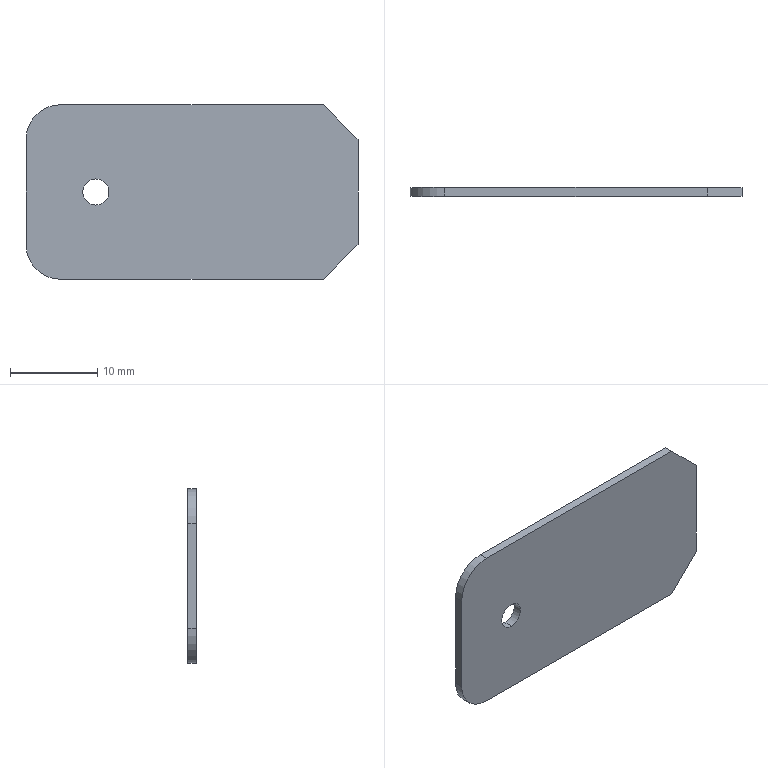Part | STEP file | RJWD-DY-0108_0003 | 1 solid | 12 faces | box 38 x 1 x 20 mm | volume 730.064 mm3 | plane 8 | cylinder 4 | commonest cylinder face diameters 3 x2 8 x2
STEP:
#1=CARTESIAN_POINT('',(0.,0.,0.));
#2=DIRECTION('',(0.,0.,1.));
#3=DIRECTION('',(1.,0.,0.));
#4=AXIS2_PLACEMENT_3D('',#1,#2,#3);
#5=CARTESIAN_POINT('',(231.,4571.8,302.644));
#6=VERTEX_POINT('',#5);
#7=CARTESIAN_POINT('',(231.,4571.8,314.644));
#8=VERTEX_POINT('',#7);
#9=CARTESIAN_POINT('',(231.,4571.8,302.644));
#10=DIRECTION('',(0.,0.,1.));
#11=VECTOR('',#10,1.);
#12=LINE('',#9,#11);
#13=CARTESIAN_POINT('',(231.,4571.8,298.644));
#14=DIRECTION('',(-1.,0.,0.));
#15=DIRECTION('',(0.,0.,-1.));
#16=AXIS2_PLACEMENT_3D('',#13,#14,#15);
#17=PLANE('',#16);
#18=CARTESIAN_POINT('',(-4.,0.));
#19=DIRECTION('',(-1.,0.));
#20=VECTOR('',#19,1.);
#21=LINE('',#18,#20);
#22=(GEOMETRIC_REPRESENTATION_CONTEXT(2)PARAMETRIC_REPRESENTATION_CONTEXT()REPRESENTATION_CONTEXT('',''));
#23=DEFINITIONAL_REPRESENTATION('',(#21),#22);
#24=PCURVE('',#17,#23);
#25=CARTESIAN_POINT('',(195.,4571.8,314.644));
#26=DIRECTION('',(0.,1.,0.));
#27=DIRECTION('',(0.,0.,1.));
#28=AXIS2_PLACEMENT_3D('',#25,#26,#27);
#29=PLANE('',#28);
#30=CARTESIAN_POINT('',(-12.,36.));
#31=DIRECTION('',(1.,0.));
#32=VECTOR('',#31,1.);
#33=LINE('',#30,#32);
#34=(GEOMETRIC_REPRESENTATION_CONTEXT(2)PARAMETRIC_REPRESENTATION_CONTEXT()REPRESENTATION_CONTEXT('',''));
#35=DEFINITIONAL_REPRESENTATION('',(#33),#34);
#36=PCURVE('',#29,#35);
#37=SURFACE_CURVE('',#12,(#24,#36),.PCURVE_S1.);
#38=EDGE_CURVE('',#6,#8,#37,.T.);
#39=ORIENTED_EDGE('',*,*,#38,.F.);
#40=CARTESIAN_POINT('',(231.,4570.8,302.644));
#41=VERTEX_POINT('',#40);
#42=CARTESIAN_POINT('',(231.,4571.8,302.644));
#43=DIRECTION('',(0.,-1.,0.));
#44=VECTOR('',#43,1.);
#45=LINE('',#42,#44);
#46=CARTESIAN_POINT('',(-4.,0.));
#47=DIRECTION('',(0.,1.));
#48=VECTOR('',#47,1.);
#49=LINE('',#46,#48);
#50=(GEOMETRIC_REPRESENTATION_CONTEXT(2)PARAMETRIC_REPRESENTATION_CONTEXT()REPRESENTATION_CONTEXT('',''));
#51=DEFINITIONAL_REPRESENTATION('',(#49),#50);
#52=PCURVE('',#17,#51);
#53=CARTESIAN_POINT('',(231.,4571.8,302.644));
#54=DIRECTION('',(-0.7071,0.,0.7071));
#55=DIRECTION('',(0.,-1.,0.));
#56=AXIS2_PLACEMENT_3D('',#53,#54,#55);
#57=PLANE('',#56);
#58=CARTESIAN_POINT('',(0.,0.));
#59=DIRECTION('',(1.,0.));
#60=VECTOR('',#59,1.);
#61=LINE('',#58,#60);
#62=(GEOMETRIC_REPRESENTATION_CONTEXT(2)PARAMETRIC_REPRESENTATION_CONTEXT()REPRESENTATION_CONTEXT('',''));
#63=DEFINITIONAL_REPRESENTATION('',(#61),#62);
#64=PCURVE('',#57,#63);
#65=SURFACE_CURVE('',#45,(#52,#64),.PCURVE_S1.);
#66=EDGE_CURVE('',#6,#41,#65,.T.);
#67=ORIENTED_EDGE('',*,*,#66,.T.);
#68=CARTESIAN_POINT('',(231.,4570.8,314.644));
#69=VERTEX_POINT('',#68);
#70=CARTESIAN_POINT('',(231.,4570.8,302.644));
#71=DIRECTION('',(0.,0.,1.));
#72=VECTOR('',#71,1.);
#73=LINE('',#70,#72);
#74=CARTESIAN_POINT('',(-4.,1.));
#75=DIRECTION('',(-1.,0.));
#76=VECTOR('',#75,1.);
#77=LINE('',#74,#76);
#78=(GEOMETRIC_REPRESENTATION_CONTEXT(2)PARAMETRIC_REPRESENTATION_CONTEXT()REPRESENTATION_CONTEXT('',''));
#79=DEFINITIONAL_REPRESENTATION('',(#77),#78);
#80=PCURVE('',#17,#79);
#81=CARTESIAN_POINT('',(195.,4570.8,314.644));
#82=DIRECTION('',(0.,1.,0.));
#83=DIRECTION('',(0.,0.,1.));
#84=AXIS2_PLACEMENT_3D('',#81,#82,#83);
#85=PLANE('',#84);
#86=CARTESIAN_POINT('',(-12.,36.));
#87=DIRECTION('',(1.,0.));
#88=VECTOR('',#87,1.);
#89=LINE('',#86,#88);
#90=(GEOMETRIC_REPRESENTATION_CONTEXT(2)PARAMETRIC_REPRESENTATION_CONTEXT()REPRESENTATION_CONTEXT('',''));
#91=DEFINITIONAL_REPRESENTATION('',(#89),#90);
#92=PCURVE('',#85,#91);
#93=SURFACE_CURVE('',#73,(#80,#92),.PCURVE_S1.);
#94=EDGE_CURVE('',#41,#69,#93,.T.);
#95=ORIENTED_EDGE('',*,*,#94,.T.);
#96=CARTESIAN_POINT('',(231.,4570.8,314.644));
#97=DIRECTION('',(0.,1.,0.));
#98=VECTOR('',#97,1.);
#99=LINE('',#96,#98);
#100=CARTESIAN_POINT('',(-16.,1.));
#101=DIRECTION('',(0.,-1.));
#102=VECTOR('',#101,1.);
#103=LINE('',#100,#102);
#104=(GEOMETRIC_REPRESENTATION_CONTEXT(2)PARAMETRIC_REPRESENTATION_CONTEXT()REPRESENTATION_CONTEXT('',''));
#105=DEFINITIONAL_REPRESENTATION('',(#103),#104);
#106=PCURVE('',#17,#105);
#107=CARTESIAN_POINT('',(227.,4571.8,318.644));
#108=DIRECTION('',(-0.7071,0.,-0.7071));
#109=DIRECTION('',(0.,-1.,0.));
#110=AXIS2_PLACEMENT_3D('',#107,#108,#109);
#111=PLANE('',#110);
#112=CARTESIAN_POINT('',(1.,-5.657));
#113=DIRECTION('',(-1.,0.));
#114=VECTOR('',#113,1.);
#115=LINE('',#112,#114);
#116=(GEOMETRIC_REPRESENTATION_CONTEXT(2)PARAMETRIC_REPRESENTATION_CONTEXT()REPRESENTATION_CONTEXT('',''));
#117=DEFINITIONAL_REPRESENTATION('',(#115),#116);
#118=PCURVE('',#111,#117);
#119=SURFACE_CURVE('',#99,(#106,#118),.PCURVE_S1.);
#120=EDGE_CURVE('',#69,#8,#119,.T.);
#121=ORIENTED_EDGE('',*,*,#120,.T.);
#122=EDGE_LOOP('',(#39,#67,#95,#121));
#123=FACE_BOUND('',#122,.F.);
#124=ADVANCED_FACE('',(#123),#17,.F.);
#125=CARTESIAN_POINT('',(193.,4571.8,314.644));
#126=VERTEX_POINT('',#125);
#127=CARTESIAN_POINT('',(197.,4571.8,318.644));
#128=VERTEX_POINT('',#127);
#129=CARTESIAN_POINT('',(197.,4571.8,314.644));
#130=DIRECTION('',(0.,1.,0.));
#131=DIRECTION('',(-1.,0.,0.));
#132=AXIS2_PLACEMENT_3D('',#129,#130,#131);
#133=CIRCLE('',#132,4.);
#134=CARTESIAN_POINT('',(0.,2.));
#135=DIRECTION('',(0.,-1.));
#136=AXIS2_PLACEMENT_2D('',#134,#135);
#137=CIRCLE('',#136,4.);
#138=(GEOMETRIC_REPRESENTATION_CONTEXT(2)PARAMETRIC_REPRESENTATION_CONTEXT()REPRESENTATION_CONTEXT('',''));
#139=DEFINITIONAL_REPRESENTATION('',(#137),#138);
#140=PCURVE('',#29,#139);
#141=CARTESIAN_POINT('',(197.,4576.711,314.644));
#142=DIRECTION('',(0.,-1.,0.));
#143=DIRECTION('',(0.,0.,1.));
#144=AXIS2_PLACEMENT_3D('',#141,#142,#143);
#145=CYLINDRICAL_SURFACE('',#144,4.);
#146=CARTESIAN_POINT('',(1.571,4.911));
#147=DIRECTION('',(-1.,0.));
#148=VECTOR('',#147,1.);
#149=LINE('',#146,#148);
#150=(GEOMETRIC_REPRESENTATION_CONTEXT(2)PARAMETRIC_REPRESENTATION_CONTEXT()REPRESENTATION_CONTEXT('',''));
#151=DEFINITIONAL_REPRESENTATION('',(#149),#150);
#152=PCURVE('',#145,#151);
#153=SURFACE_CURVE('',#133,(#140,#152),.PCURVE_S1.);
#154=EDGE_CURVE('',#126,#128,#153,.T.);
#155=ORIENTED_EDGE('',*,*,#154,.F.);
#156=CARTESIAN_POINT('',(193.,4571.8,302.644));
#157=VERTEX_POINT('',#156);
#158=CARTESIAN_POINT('',(193.,4571.8,314.644));
#159=DIRECTION('',(0.,0.,-1.));
#160=VECTOR('',#159,1.);
#161=LINE('',#158,#160);
#162=CARTESIAN_POINT('',(0.,-2.));
#163=DIRECTION('',(-1.,0.));
#164=VECTOR('',#163,1.);
#165=LINE('',#162,#164);
#166=(GEOMETRIC_REPRESENTATION_CONTEXT(2)PARAMETRIC_REPRESENTATION_CONTEXT()REPRESENTATION_CONTEXT('',''));
#167=DEFINITIONAL_REPRESENTATION('',(#165),#166);
#168=PCURVE('',#29,#167);
#169=CARTESIAN_POINT('',(193.,4571.8,314.644));
#170=DIRECTION('',(1.,0.,0.));
#171=DIRECTION('',(0.,0.,1.));
#172=AXIS2_PLACEMENT_3D('',#169,#170,#171);
#173=PLANE('',#172);
#174=CARTESIAN_POINT('',(0.,0.));
#175=DIRECTION('',(-1.,0.));
#176=VECTOR('',#175,1.);
#177=LINE('',#174,#176);
#178=(GEOMETRIC_REPRESENTATION_CONTEXT(2)PARAMETRIC_REPRESENTATION_CONTEXT()REPRESENTATION_CONTEXT('',''));
#179=DEFINITIONAL_REPRESENTATION('',(#177),#178);
#180=PCURVE('',#173,#179);
#181=SURFACE_CURVE('',#161,(#168,#180),.PCURVE_S1.);
#182=EDGE_CURVE('',#126,#157,#181,.T.);
#183=ORIENTED_EDGE('',*,*,#182,.T.);
#184=CARTESIAN_POINT('',(197.,4571.8,298.644));
#185=VERTEX_POINT('',#184);
#186=CARTESIAN_POINT('',(197.,4571.8,302.644));
#187=DIRECTION('',(0.,1.,0.));
#188=DIRECTION('',(0.,0.,-1.));
#189=AXIS2_PLACEMENT_3D('',#186,#187,#188);
#190=CIRCLE('',#189,4.);
#191=CARTESIAN_POINT('',(-12.,2.));
#192=DIRECTION('',(-1.,0.));
#193=AXIS2_PLACEMENT_2D('',#191,#192);
#194=CIRCLE('',#193,4.);
#195=(GEOMETRIC_REPRESENTATION_CONTEXT(2)PARAMETRIC_REPRESENTATION_CONTEXT()REPRESENTATION_CONTEXT('',''));
#196=DEFINITIONAL_REPRESENTATION('',(#194),#195);
#197=PCURVE('',#29,#196);
#198=CARTESIAN_POINT('',(197.,4576.711,302.644));
#199=DIRECTION('',(0.,-1.,0.));
#200=DIRECTION('',(-1.,0.,0.));
#201=AXIS2_PLACEMENT_3D('',#198,#199,#200);
#202=CYLINDRICAL_SURFACE('',#201,4.);
#203=CARTESIAN_POINT('',(1.571,4.911));
#204=DIRECTION('',(-1.,0.));
#205=VECTOR('',#204,1.);
#206=LINE('',#203,#205);
#207=(GEOMETRIC_REPRESENTATION_CONTEXT(2)PARAMETRIC_REPRESENTATION_CONTEXT()REPRESENTATION_CONTEXT('',''));
#208=DEFINITIONAL_REPRESENTATION('',(#206),#207);
#209=PCURVE('',#202,#208);
#210=SURFACE_CURVE('',#190,(#197,#209),.PCURVE_S1.);
#211=EDGE_CURVE('',#185,#157,#210,.T.);
#212=ORIENTED_EDGE('',*,*,#211,.F.);
#213=CARTESIAN_POINT('',(227.,4571.8,298.644));
#214=VERTEX_POINT('',#213);
#215=CARTESIAN_POINT('',(227.,4571.8,298.644));
#216=DIRECTION('',(-1.,0.,0.));
#217=VECTOR('',#216,1.);
#218=LINE('',#215,#217);
#219=CARTESIAN_POINT('',(-16.,32.));
#220=DIRECTION('',(0.,-1.));
#221=VECTOR('',#220,1.);
#222=LINE('',#219,#221);
#223=(GEOMETRIC_REPRESENTATION_CONTEXT(2)PARAMETRIC_REPRESENTATION_CONTEXT()REPRESENTATION_CONTEXT('',''));
#224=DEFINITIONAL_REPRESENTATION('',(#222),#223);
#225=PCURVE('',#29,#224);
#226=CARTESIAN_POINT('',(195.,4571.8,298.644));
#227=DIRECTION('',(0.,0.,1.));
#228=DIRECTION('',(-1.,0.,0.));
#229=AXIS2_PLACEMENT_3D('',#226,#227,#228);
#230=PLANE('',#229);
#231=CARTESIAN_POINT('',(-32.,0.));
#232=DIRECTION('',(1.,0.));
#233=VECTOR('',#232,1.);
#234=LINE('',#231,#233);
#235=(GEOMETRIC_REPRESENTATION_CONTEXT(2)PARAMETRIC_REPRESENTATION_CONTEXT()REPRESENTATION_CONTEXT('',''));
#236=DEFINITIONAL_REPRESENTATION('',(#234),#235);
#237=PCURVE('',#230,#236);
#238=SURFACE_CURVE('',#218,(#225,#237),.PCURVE_S1.);
#239=EDGE_CURVE('',#214,#185,#238,.T.);
#240=ORIENTED_EDGE('',*,*,#239,.F.);
#241=CARTESIAN_POINT('',(231.,4571.8,302.644));
#242=DIRECTION('',(-0.7071,0.,-0.7071));
#243=VECTOR('',#242,1.);
#244=LINE('',#241,#243);
#245=CARTESIAN_POINT('',(-12.,36.));
#246=DIRECTION('',(-0.7071,-0.7071));
#247=VECTOR('',#246,1.);
#248=LINE('',#245,#247);
#249=(GEOMETRIC_REPRESENTATION_CONTEXT(2)PARAMETRIC_REPRESENTATION_CONTEXT()REPRESENTATION_CONTEXT('',''));
#250=DEFINITIONAL_REPRESENTATION('',(#248),#249);
#251=PCURVE('',#29,#250);
#252=CARTESIAN_POINT('',(0.,0.));
#253=DIRECTION('',(0.,-1.));
#254=VECTOR('',#253,1.);
#255=LINE('',#252,#254);
#256=(GEOMETRIC_REPRESENTATION_CONTEXT(2)PARAMETRIC_REPRESENTATION_CONTEXT()REPRESENTATION_CONTEXT('',''));
#257=DEFINITIONAL_REPRESENTATION('',(#255),#256);
#258=PCURVE('',#57,#257);
#259=SURFACE_CURVE('',#244,(#251,#258),.PCURVE_S1.);
#260=EDGE_CURVE('',#6,#214,#259,.T.);
#261=ORIENTED_EDGE('',*,*,#260,.F.);
#262=ORIENTED_EDGE('',*,*,#38,.T.);
#263=CARTESIAN_POINT('',(227.,4571.8,318.644));
#264=VERTEX_POINT('',#263);
#265=CARTESIAN_POINT('',(227.,4571.8,318.644));
#266=DIRECTION('',(0.7071,0.,-0.7071));
#267=VECTOR('',#266,1.);
#268=LINE('',#265,#267);
#269=CARTESIAN_POINT('',(4.,32.));
#270=DIRECTION('',(-0.7071,0.7071));
#271=VECTOR('',#270,1.);
#272=LINE('',#269,#271);
#273=(GEOMETRIC_REPRESENTATION_CONTEXT(2)PARAMETRIC_REPRESENTATION_CONTEXT()REPRESENTATION_CONTEXT('',''));
#274=DEFINITIONAL_REPRESENTATION('',(#272),#273);
#275=PCURVE('',#29,#274);
#276=CARTESIAN_POINT('',(0.,0.));
#277=DIRECTION('',(0.,-1.));
#278=VECTOR('',#277,1.);
#279=LINE('',#276,#278);
#280=(GEOMETRIC_REPRESENTATION_CONTEXT(2)PARAMETRIC_REPRESENTATION_CONTEXT()REPRESENTATION_CONTEXT('',''));
#281=DEFINITIONAL_REPRESENTATION('',(#279),#280);
#282=PCURVE('',#111,#281);
#283=SURFACE_CURVE('',#268,(#275,#282),.PCURVE_S1.);
#284=EDGE_CURVE('',#264,#8,#283,.T.);
#285=ORIENTED_EDGE('',*,*,#284,.F.);
#286=CARTESIAN_POINT('',(197.,4571.8,318.644));
#287=DIRECTION('',(1.,0.,0.));
#288=VECTOR('',#287,1.);
#289=LINE('',#286,#288);
#290=CARTESIAN_POINT('',(4.,2.));
#291=DIRECTION('',(0.,1.));
#292=VECTOR('',#291,1.);
#293=LINE('',#290,#292);
#294=(GEOMETRIC_REPRESENTATION_CONTEXT(2)PARAMETRIC_REPRESENTATION_CONTEXT()REPRESENTATION_CONTEXT('',''));
#295=DEFINITIONAL_REPRESENTATION('',(#293),#294);
#296=PCURVE('',#29,#295);
#297=CARTESIAN_POINT('',(231.,4571.8,318.644));
#298=DIRECTION('',(0.,0.,-1.));
#299=DIRECTION('',(1.,0.,0.));
#300=AXIS2_PLACEMENT_3D('',#297,#298,#299);
#301=PLANE('',#300);
#302=CARTESIAN_POINT('',(-34.,0.));
#303=DIRECTION('',(1.,0.));
#304=VECTOR('',#303,1.);
#305=LINE('',#302,#304);
#306=(GEOMETRIC_REPRESENTATION_CONTEXT(2)PARAMETRIC_REPRESENTATION_CONTEXT()REPRESENTATION_CONTEXT('',''));
#307=DEFINITIONAL_REPRESENTATION('',(#305),#306);
#308=PCURVE('',#301,#307);
#309=SURFACE_CURVE('',#289,(#296,#308),.PCURVE_S1.);
#310=EDGE_CURVE('',#128,#264,#309,.T.);
#311=ORIENTED_EDGE('',*,*,#310,.F.);
#312=EDGE_LOOP('',(#155,#183,#212,#240,#261,#262,#285,#311));
#313=FACE_BOUND('',#312,.F.);
#314=CARTESIAN_POINT('',(200.999,4571.8,310.144));
#315=VERTEX_POINT('',#314);
#316=CARTESIAN_POINT('',(200.999,4571.8,307.144));
#317=VERTEX_POINT('',#316);
#318=CARTESIAN_POINT('',(200.999,4571.8,308.644));
#319=DIRECTION('',(0.,1.,0.));
#320=DIRECTION('',(0.,0.,1.));
#321=AXIS2_PLACEMENT_3D('',#318,#319,#320);
#322=CIRCLE('',#321,1.5);
#323=CARTESIAN_POINT('',(-6.,5.999));
#324=DIRECTION('',(1.,0.));
#325=AXIS2_PLACEMENT_2D('',#323,#324);
#326=CIRCLE('',#325,1.5);
#327=(GEOMETRIC_REPRESENTATION_CONTEXT(2)PARAMETRIC_REPRESENTATION_CONTEXT()REPRESENTATION_CONTEXT('',''));
#328=DEFINITIONAL_REPRESENTATION('',(#326),#327);
#329=PCURVE('',#29,#328);
#330=CARTESIAN_POINT('',(200.999,4571.8,308.644));
#331=DIRECTION('',(0.,-1.,0.));
#332=DIRECTION('',(0.,0.,-1.));
#333=AXIS2_PLACEMENT_3D('',#330,#331,#332);
#334=CYLINDRICAL_SURFACE('',#333,1.5);
#335=CARTESIAN_POINT('',(3.142,0.));
#336=DIRECTION('',(-1.,0.));
#337=VECTOR('',#336,1.);
#338=LINE('',#335,#337);
#339=(GEOMETRIC_REPRESENTATION_CONTEXT(2)PARAMETRIC_REPRESENTATION_CONTEXT()REPRESENTATION_CONTEXT('',''));
#340=DEFINITIONAL_REPRESENTATION('',(#338),#339);
#341=PCURVE('',#334,#340);
#342=SURFACE_CURVE('',#322,(#329,#341),.PCURVE_S1.);
#343=EDGE_CURVE('',#315,#317,#342,.T.);
#344=ORIENTED_EDGE('',*,*,#343,.T.);
#345=CARTESIAN_POINT('',(200.999,4571.8,308.644));
#346=DIRECTION('',(0.,-1.,0.));
#347=DIRECTION('',(0.,0.,1.));
#348=AXIS2_PLACEMENT_3D('',#345,#346,#347);
#349=CIRCLE('',#348,1.5);
#350=CARTESIAN_POINT('',(-4.5,5.999));
#351=CARTESIAN_POINT('',(-4.5,3.401));
#352=CARTESIAN_POINT('',(-6.75,4.7));
#353=CARTESIAN_POINT('',(-9.,5.999));
#354=CARTESIAN_POINT('',(-6.75,7.298));
#355=CARTESIAN_POINT('',(-4.5,8.597));
#356=CARTESIAN_POINT('',(-4.5,5.999));
#357=(BOUNDED_CURVE()B_SPLINE_CURVE(2,(#350,#351,#352,#353,#354,#355,#356),.UNSPECIFIED.,.T.,.F.)B_SPLINE_CURVE_WITH_KNOTS((1,2,2,2,2,1),(-2.094,0.,2.094,4.189,6.283,8.378),.UNSPECIFIED.)CURVE()GEOMETRIC_REPRESENTATION_ITEM()RATIONAL_B_SPLINE_CURVE((1.,0.5,1.,0.5,1.,0.5,1.))REPRESENTATION_ITEM(''));
#358=(GEOMETRIC_REPRESENTATION_CONTEXT(2)PARAMETRIC_REPRESENTATION_CONTEXT()REPRESENTATION_CONTEXT('',''));
#359=DEFINITIONAL_REPRESENTATION('',(#357),#358);
#360=PCURVE('',#29,#359);
#361=CARTESIAN_POINT('',(200.999,4571.8,308.644));
#362=DIRECTION('',(0.,-1.,0.));
#363=DIRECTION('',(0.,0.,-1.));
#364=AXIS2_PLACEMENT_3D('',#361,#362,#363);
#365=CYLINDRICAL_SURFACE('',#364,1.5);
#366=CARTESIAN_POINT('',(3.142,0.));
#367=DIRECTION('',(1.,0.));
#368=VECTOR('',#367,1.);
#369=LINE('',#366,#368);
#370=(GEOMETRIC_REPRESENTATION_CONTEXT(2)PARAMETRIC_REPRESENTATION_CONTEXT()REPRESENTATION_CONTEXT('',''));
#371=DEFINITIONAL_REPRESENTATION('',(#369),#370);
#372=PCURVE('',#365,#371);
#373=SURFACE_CURVE('',#349,(#360,#372),.PCURVE_S1.);
#374=EDGE_CURVE('',#315,#317,#373,.T.);
#375=ORIENTED_EDGE('',*,*,#374,.F.);
#376=EDGE_LOOP('',(#344,#375));
#377=FACE_BOUND('',#376,.F.);
#378=ADVANCED_FACE('',(#313,#377),#29,.T.);
#379=ORIENTED_EDGE('',*,*,#343,.F.);
#380=CARTESIAN_POINT('',(200.999,4570.8,310.144));
#381=VERTEX_POINT('',#380);
#382=CARTESIAN_POINT('',(200.999,4571.8,310.144));
#383=DIRECTION('',(0.,-1.,0.));
#384=VECTOR('',#383,1.);
#385=LINE('',#382,#384);
#386=CARTESIAN_POINT('',(3.142,0.));
#387=DIRECTION('',(0.,1.));
#388=VECTOR('',#387,1.);
#389=LINE('',#386,#388);
#390=(GEOMETRIC_REPRESENTATION_CONTEXT(2)PARAMETRIC_REPRESENTATION_CONTEXT()REPRESENTATION_CONTEXT('',''));
#391=DEFINITIONAL_REPRESENTATION('',(#389),#390);
#392=PCURVE('',#334,#391);
#393=CARTESIAN_POINT('',(3.142,0.));
#394=DIRECTION('',(0.,1.));
#395=VECTOR('',#394,1.);
#396=LINE('',#393,#395);
#397=(GEOMETRIC_REPRESENTATION_CONTEXT(2)PARAMETRIC_REPRESENTATION_CONTEXT()REPRESENTATION_CONTEXT('',''));
#398=DEFINITIONAL_REPRESENTATION('',(#396),#397);
#399=PCURVE('',#365,#398);
#400=SURFACE_CURVE('',#385,(#392,#399),.PCURVE_S1.);
#401=EDGE_CURVE('',#315,#381,#400,.T.);
#402=ORIENTED_EDGE('',*,*,#401,.T.);
#403=CARTESIAN_POINT('',(200.999,4570.8,307.144));
#404=VERTEX_POINT('',#403);
#405=CARTESIAN_POINT('',(200.999,4570.8,308.644));
#406=DIRECTION('',(0.,-1.,0.));
#407=DIRECTION('',(0.,0.,-1.));
#408=AXIS2_PLACEMENT_3D('',#405,#406,#407);
#409=CIRCLE('',#408,1.5);
#410=CARTESIAN_POINT('',(0.,1.));
#411=DIRECTION('',(1.,0.));
#412=VECTOR('',#411,1.);
#413=LINE('',#410,#412);
#414=(GEOMETRIC_REPRESENTATION_CONTEXT(2)PARAMETRIC_REPRESENTATION_CONTEXT()REPRESENTATION_CONTEXT('',''));
#415=DEFINITIONAL_REPRESENTATION('',(#413),#414);
#416=PCURVE('',#334,#415);
#417=CARTESIAN_POINT('',(-7.5,5.999));
#418=CARTESIAN_POINT('',(-7.5,8.597));
#419=CARTESIAN_POINT('',(-5.25,7.298));
#420=CARTESIAN_POINT('',(-3.,5.999));
#421=CARTESIAN_POINT('',(-5.25,4.7));
#422=CARTESIAN_POINT('',(-7.5,3.401));
#423=CARTESIAN_POINT('',(-7.5,5.999));
#424=(BOUNDED_CURVE()B_SPLINE_CURVE(2,(#417,#418,#419,#420,#421,#422,#423),.UNSPECIFIED.,.T.,.F.)B_SPLINE_CURVE_WITH_KNOTS((1,2,2,2,2,1),(-2.094,0.,2.094,4.189,6.283,8.378),.UNSPECIFIED.)CURVE()GEOMETRIC_REPRESENTATION_ITEM()RATIONAL_B_SPLINE_CURVE((1.,0.5,1.,0.5,1.,0.5,1.))REPRESENTATION_ITEM(''));
#425=(GEOMETRIC_REPRESENTATION_CONTEXT(2)PARAMETRIC_REPRESENTATION_CONTEXT()REPRESENTATION_CONTEXT('',''));
#426=DEFINITIONAL_REPRESENTATION('',(#424),#425);
#427=PCURVE('',#85,#426);
#428=SURFACE_CURVE('',#409,(#416,#427),.PCURVE_S1.);
#429=EDGE_CURVE('',#404,#381,#428,.T.);
#430=ORIENTED_EDGE('',*,*,#429,.F.);
#431=CARTESIAN_POINT('',(200.999,4571.8,307.144));
#432=DIRECTION('',(0.,-1.,0.));
#433=VECTOR('',#432,1.);
#434=LINE('',#431,#433);
#435=CARTESIAN_POINT('',(0.,0.));
#436=DIRECTION('',(0.,1.));
#437=VECTOR('',#436,1.);
#438=LINE('',#435,#437);
#439=(GEOMETRIC_REPRESENTATION_CONTEXT(2)PARAMETRIC_REPRESENTATION_CONTEXT()REPRESENTATION_CONTEXT('',''));
#440=DEFINITIONAL_REPRESENTATION('',(#438),#439);
#441=PCURVE('',#334,#440);
#442=CARTESIAN_POINT('',(6.283,0.));
#443=DIRECTION('',(0.,1.));
#444=VECTOR('',#443,1.);
#445=LINE('',#442,#444);
#446=(GEOMETRIC_REPRESENTATION_CONTEXT(2)PARAMETRIC_REPRESENTATION_CONTEXT()REPRESENTATION_CONTEXT('',''));
#447=DEFINITIONAL_REPRESENTATION('',(#445),#446);
#448=PCURVE('',#365,#447);
#449=SURFACE_CURVE('',#434,(#441,#448),.PCURVE_S1.);
#450=EDGE_CURVE('',#317,#404,#449,.T.);
#451=ORIENTED_EDGE('',*,*,#450,.F.);
#452=EDGE_LOOP('',(#379,#402,#430,#451));
#453=FACE_BOUND('',#452,.F.);
#454=ADVANCED_FACE('',(#453),#334,.F.);
#455=ORIENTED_EDGE('',*,*,#374,.T.);
#456=ORIENTED_EDGE('',*,*,#450,.T.);
#457=CARTESIAN_POINT('',(200.999,4570.8,308.644));
#458=DIRECTION('',(0.,-1.,0.));
#459=DIRECTION('',(0.,0.,1.));
#460=AXIS2_PLACEMENT_3D('',#457,#458,#459);
#461=CIRCLE('',#460,1.5);
#462=CARTESIAN_POINT('',(3.142,1.));
#463=DIRECTION('',(1.,0.));
#464=VECTOR('',#463,1.);
#465=LINE('',#462,#464);
#466=(GEOMETRIC_REPRESENTATION_CONTEXT(2)PARAMETRIC_REPRESENTATION_CONTEXT()REPRESENTATION_CONTEXT('',''));
#467=DEFINITIONAL_REPRESENTATION('',(#465),#466);
#468=PCURVE('',#365,#467);
#469=CARTESIAN_POINT('',(-4.5,5.999));
#470=CARTESIAN_POINT('',(-4.5,3.401));
#471=CARTESIAN_POINT('',(-6.75,4.7));
#472=CARTESIAN_POINT('',(-9.,5.999));
#473=CARTESIAN_POINT('',(-6.75,7.298));
#474=CARTESIAN_POINT('',(-4.5,8.597));
#475=CARTESIAN_POINT('',(-4.5,5.999));
#476=(BOUNDED_CURVE()B_SPLINE_CURVE(2,(#469,#470,#471,#472,#473,#474,#475),.UNSPECIFIED.,.T.,.F.)B_SPLINE_CURVE_WITH_KNOTS((1,2,2,2,2,1),(-2.094,0.,2.094,4.189,6.283,8.378),.UNSPECIFIED.)CURVE()GEOMETRIC_REPRESENTATION_ITEM()RATIONAL_B_SPLINE_CURVE((1.,0.5,1.,0.5,1.,0.5,1.))REPRESENTATION_ITEM(''));
#477=(GEOMETRIC_REPRESENTATION_CONTEXT(2)PARAMETRIC_REPRESENTATION_CONTEXT()REPRESENTATION_CONTEXT('',''));
#478=DEFINITIONAL_REPRESENTATION('',(#476),#477);
#479=PCURVE('',#85,#478);
#480=SURFACE_CURVE('',#461,(#468,#479),.PCURVE_S1.);
#481=EDGE_CURVE('',#381,#404,#480,.T.);
#482=ORIENTED_EDGE('',*,*,#481,.F.);
#483=ORIENTED_EDGE('',*,*,#401,.F.);
#484=EDGE_LOOP('',(#455,#456,#482,#483));
#485=FACE_BOUND('',#484,.F.);
#486=ADVANCED_FACE('',(#485),#365,.F.);
#487=CARTESIAN_POINT('',(197.,4570.8,318.644));
#488=VERTEX_POINT('',#487);
#489=CARTESIAN_POINT('',(193.,4570.8,314.644));
#490=VERTEX_POINT('',#489);
#491=CARTESIAN_POINT('',(197.,4570.8,314.644));
#492=DIRECTION('',(0.,-1.,0.));
#493=DIRECTION('',(0.,0.,1.));
#494=AXIS2_PLACEMENT_3D('',#491,#492,#493);
#495=CIRCLE('',#494,4.);
#496=CARTESIAN_POINT('',(4.,2.));
#497=CARTESIAN_POINT('',(4.,-4.928));
#498=CARTESIAN_POINT('',(-2.,-1.464));
#499=CARTESIAN_POINT('',(-8.,2.));
#500=CARTESIAN_POINT('',(-2.,5.464));
#501=CARTESIAN_POINT('',(4.,8.928));
#502=CARTESIAN_POINT('',(4.,2.));
#503=(BOUNDED_CURVE()B_SPLINE_CURVE(2,(#496,#497,#498,#499,#500,#501,#502),.UNSPECIFIED.,.T.,.F.)B_SPLINE_CURVE_WITH_KNOTS((1,2,2,2,2,1),(-2.094,0.,2.094,4.189,6.283,8.378),.UNSPECIFIED.)CURVE()GEOMETRIC_REPRESENTATION_ITEM()RATIONAL_B_SPLINE_CURVE((1.,0.5,1.,0.5,1.,0.5,1.))REPRESENTATION_ITEM(''));
#504=(GEOMETRIC_REPRESENTATION_CONTEXT(2)PARAMETRIC_REPRESENTATION_CONTEXT()REPRESENTATION_CONTEXT('',''));
#505=DEFINITIONAL_REPRESENTATION('',(#503),#504);
#506=PCURVE('',#85,#505);
#507=CARTESIAN_POINT('',(0.,5.911));
#508=DIRECTION('',(1.,0.));
#509=VECTOR('',#508,1.);
#510=LINE('',#507,#509);
#511=(GEOMETRIC_REPRESENTATION_CONTEXT(2)PARAMETRIC_REPRESENTATION_CONTEXT()REPRESENTATION_CONTEXT('',''));
#512=DEFINITIONAL_REPRESENTATION('',(#510),#511);
#513=PCURVE('',#145,#512);
#514=SURFACE_CURVE('',#495,(#506,#513),.PCURVE_S1.);
#515=EDGE_CURVE('',#488,#490,#514,.T.);
#516=ORIENTED_EDGE('',*,*,#515,.F.);
#517=CARTESIAN_POINT('',(227.,4570.8,318.644));
#518=VERTEX_POINT('',#517);
#519=CARTESIAN_POINT('',(227.,4570.8,318.644));
#520=DIRECTION('',(-1.,0.,0.));
#521=VECTOR('',#520,1.);
#522=LINE('',#519,#521);
#523=CARTESIAN_POINT('',(4.,32.));
#524=DIRECTION('',(0.,-1.));
#525=VECTOR('',#524,1.);
#526=LINE('',#523,#525);
#527=(GEOMETRIC_REPRESENTATION_CONTEXT(2)PARAMETRIC_REPRESENTATION_CONTEXT()REPRESENTATION_CONTEXT('',''));
#528=DEFINITIONAL_REPRESENTATION('',(#526),#527);
#529=PCURVE('',#85,#528);
#530=CARTESIAN_POINT('',(-4.,1.));
#531=DIRECTION('',(-1.,0.));
#532=VECTOR('',#531,1.);
#533=LINE('',#530,#532);
#534=(GEOMETRIC_REPRESENTATION_CONTEXT(2)PARAMETRIC_REPRESENTATION_CONTEXT()REPRESENTATION_CONTEXT('',''));
#535=DEFINITIONAL_REPRESENTATION('',(#533),#534);
#536=PCURVE('',#301,#535);
#537=SURFACE_CURVE('',#522,(#529,#536),.PCURVE_S1.);
#538=EDGE_CURVE('',#518,#488,#537,.T.);
#539=ORIENTED_EDGE('',*,*,#538,.F.);
#540=CARTESIAN_POINT('',(231.,4570.8,314.644));
#541=DIRECTION('',(-0.7071,0.,0.7071));
#542=VECTOR('',#541,1.);
#543=LINE('',#540,#542);
#544=CARTESIAN_POINT('',(0.,36.));
#545=DIRECTION('',(0.7071,-0.7071));
#546=VECTOR('',#545,1.);
#547=LINE('',#544,#546);
#548=(GEOMETRIC_REPRESENTATION_CONTEXT(2)PARAMETRIC_REPRESENTATION_CONTEXT()REPRESENTATION_CONTEXT('',''));
#549=DEFINITIONAL_REPRESENTATION('',(#547),#548);
#550=PCURVE('',#85,#549);
#551=CARTESIAN_POINT('',(1.,-5.657));
#552=DIRECTION('',(0.,1.));
#553=VECTOR('',#552,1.);
#554=LINE('',#551,#553);
#555=(GEOMETRIC_REPRESENTATION_CONTEXT(2)PARAMETRIC_REPRESENTATION_CONTEXT()REPRESENTATION_CONTEXT('',''));
#556=DEFINITIONAL_REPRESENTATION('',(#554),#555);
#557=PCURVE('',#111,#556);
#558=SURFACE_CURVE('',#543,(#550,#557),.PCURVE_S1.);
#559=EDGE_CURVE('',#69,#518,#558,.T.);
#560=ORIENTED_EDGE('',*,*,#559,.F.);
#561=ORIENTED_EDGE('',*,*,#94,.F.);
#562=CARTESIAN_POINT('',(227.,4570.8,298.644));
#563=VERTEX_POINT('',#562);
#564=CARTESIAN_POINT('',(227.,4570.8,298.644));
#565=DIRECTION('',(0.7071,0.,0.7071));
#566=VECTOR('',#565,1.);
#567=LINE('',#564,#566);
#568=CARTESIAN_POINT('',(-16.,32.));
#569=DIRECTION('',(0.7071,0.7071));
#570=VECTOR('',#569,1.);
#571=LINE('',#568,#570);
#572=(GEOMETRIC_REPRESENTATION_CONTEXT(2)PARAMETRIC_REPRESENTATION_CONTEXT()REPRESENTATION_CONTEXT('',''));
#573=DEFINITIONAL_REPRESENTATION('',(#571),#572);
#574=PCURVE('',#85,#573);
#575=CARTESIAN_POINT('',(1.,-5.657));
#576=DIRECTION('',(0.,1.));
#577=VECTOR('',#576,1.);
#578=LINE('',#575,#577);
#579=(GEOMETRIC_REPRESENTATION_CONTEXT(2)PARAMETRIC_REPRESENTATION_CONTEXT()REPRESENTATION_CONTEXT('',''));
#580=DEFINITIONAL_REPRESENTATION('',(#578),#579);
#581=PCURVE('',#57,#580);
#582=SURFACE_CURVE('',#567,(#574,#581),.PCURVE_S1.);
#583=EDGE_CURVE('',#563,#41,#582,.T.);
#584=ORIENTED_EDGE('',*,*,#583,.F.);
#585=CARTESIAN_POINT('',(197.,4570.8,298.644));
#586=VERTEX_POINT('',#585);
#587=CARTESIAN_POINT('',(197.,4570.8,298.644));
#588=DIRECTION('',(1.,0.,0.));
#589=VECTOR('',#588,1.);
#590=LINE('',#587,#589);
#591=CARTESIAN_POINT('',(-16.,2.));
#592=DIRECTION('',(0.,1.));
#593=VECTOR('',#592,1.);
#594=LINE('',#591,#593);
#595=(GEOMETRIC_REPRESENTATION_CONTEXT(2)PARAMETRIC_REPRESENTATION_CONTEXT()REPRESENTATION_CONTEXT('',''));
#596=DEFINITIONAL_REPRESENTATION('',(#594),#595);
#597=PCURVE('',#85,#596);
#598=CARTESIAN_POINT('',(-2.,1.));
#599=DIRECTION('',(-1.,0.));
#600=VECTOR('',#599,1.);
#601=LINE('',#598,#600);
#602=(GEOMETRIC_REPRESENTATION_CONTEXT(2)PARAMETRIC_REPRESENTATION_CONTEXT()REPRESENTATION_CONTEXT('',''));
#603=DEFINITIONAL_REPRESENTATION('',(#601),#602);
#604=PCURVE('',#230,#603);
#605=SURFACE_CURVE('',#590,(#597,#604),.PCURVE_S1.);
#606=EDGE_CURVE('',#586,#563,#605,.T.);
#607=ORIENTED_EDGE('',*,*,#606,.F.);
#608=CARTESIAN_POINT('',(193.,4570.8,302.644));
#609=VERTEX_POINT('',#608);
#610=CARTESIAN_POINT('',(197.,4570.8,302.644));
#611=DIRECTION('',(0.,-1.,0.));
#612=DIRECTION('',(-1.,0.,0.));
#613=AXIS2_PLACEMENT_3D('',#610,#611,#612);
#614=CIRCLE('',#613,4.);
#615=CARTESIAN_POINT('',(-12.,-2.));
#616=CARTESIAN_POINT('',(-18.928,-2.));
#617=CARTESIAN_POINT('',(-15.464,4.));
#618=CARTESIAN_POINT('',(-12.,10.));
#619=CARTESIAN_POINT('',(-8.536,4.));
#620=CARTESIAN_POINT('',(-5.072,-2.));
#621=CARTESIAN_POINT('',(-12.,-2.));
#622=(BOUNDED_CURVE()B_SPLINE_CURVE(2,(#615,#616,#617,#618,#619,#620,#621),.UNSPECIFIED.,.T.,.F.)B_SPLINE_CURVE_WITH_KNOTS((1,2,2,2,2,1),(-2.094,0.,2.094,4.189,6.283,8.378),.UNSPECIFIED.)CURVE()GEOMETRIC_REPRESENTATION_ITEM()RATIONAL_B_SPLINE_CURVE((1.,0.5,1.,0.5,1.,0.5,1.))REPRESENTATION_ITEM(''));
#623=(GEOMETRIC_REPRESENTATION_CONTEXT(2)PARAMETRIC_REPRESENTATION_CONTEXT()REPRESENTATION_CONTEXT('',''));
#624=DEFINITIONAL_REPRESENTATION('',(#622),#623);
#625=PCURVE('',#85,#624);
#626=CARTESIAN_POINT('',(0.,5.911));
#627=DIRECTION('',(1.,0.));
#628=VECTOR('',#627,1.);
#629=LINE('',#626,#628);
#630=(GEOMETRIC_REPRESENTATION_CONTEXT(2)PARAMETRIC_REPRESENTATION_CONTEXT()REPRESENTATION_CONTEXT('',''));
#631=DEFINITIONAL_REPRESENTATION('',(#629),#630);
#632=PCURVE('',#202,#631);
#633=SURFACE_CURVE('',#614,(#625,#632),.PCURVE_S1.);
#634=EDGE_CURVE('',#609,#586,#633,.T.);
#635=ORIENTED_EDGE('',*,*,#634,.F.);
#636=CARTESIAN_POINT('',(193.,4570.8,314.644));
#637=DIRECTION('',(0.,0.,-1.));
#638=VECTOR('',#637,1.);
#639=LINE('',#636,#638);
#640=CARTESIAN_POINT('',(0.,-2.));
#641=DIRECTION('',(-1.,0.));
#642=VECTOR('',#641,1.);
#643=LINE('',#640,#642);
#644=(GEOMETRIC_REPRESENTATION_CONTEXT(2)PARAMETRIC_REPRESENTATION_CONTEXT()REPRESENTATION_CONTEXT('',''));
#645=DEFINITIONAL_REPRESENTATION('',(#643),#644);
#646=PCURVE('',#85,#645);
#647=CARTESIAN_POINT('',(0.,1.));
#648=DIRECTION('',(-1.,0.));
#649=VECTOR('',#648,1.);
#650=LINE('',#647,#649);
#651=(GEOMETRIC_REPRESENTATION_CONTEXT(2)PARAMETRIC_REPRESENTATION_CONTEXT()REPRESENTATION_CONTEXT('',''));
#652=DEFINITIONAL_REPRESENTATION('',(#650),#651);
#653=PCURVE('',#173,#652);
#654=SURFACE_CURVE('',#639,(#646,#653),.PCURVE_S1.);
#655=EDGE_CURVE('',#490,#609,#654,.T.);
#656=ORIENTED_EDGE('',*,*,#655,.F.);
#657=EDGE_LOOP('',(#516,#539,#560,#561,#584,#607,#635,#656));
#658=FACE_BOUND('',#657,.F.);
#659=ORIENTED_EDGE('',*,*,#429,.T.);
#660=ORIENTED_EDGE('',*,*,#481,.T.);
#661=EDGE_LOOP('',(#659,#660));
#662=FACE_BOUND('',#661,.F.);
#663=ADVANCED_FACE('',(#658,#662),#85,.F.);
#664=CARTESIAN_POINT('',(197.,4571.8,318.644));
#665=DIRECTION('',(0.,-1.,0.));
#666=VECTOR('',#665,1.);
#667=LINE('',#664,#666);
#668=CARTESIAN_POINT('',(0.,4.911));
#669=CARTESIAN_POINT('',(0.,4.926));
#670=CARTESIAN_POINT('',(0.,4.956));
#671=CARTESIAN_POINT('',(0.,5.002));
#672=CARTESIAN_POINT('',(0.,5.047));
#673=CARTESIAN_POINT('',(0.,5.093));
#674=CARTESIAN_POINT('',(0.,5.138));
#675=CARTESIAN_POINT('',(0.,5.184));
#676=CARTESIAN_POINT('',(0.,5.229));
#677=CARTESIAN_POINT('',(0.,5.274));
#678=CARTESIAN_POINT('',(0.,5.32));
#679=CARTESIAN_POINT('',(0.,5.365));
#680=CARTESIAN_POINT('',(0.,5.411));
#681=CARTESIAN_POINT('',(0.,5.456));
#682=CARTESIAN_POINT('',(0.,5.502));
#683=CARTESIAN_POINT('',(0.,5.547));
#684=CARTESIAN_POINT('',(0.,5.593));
#685=CARTESIAN_POINT('',(0.,5.638));
#686=CARTESIAN_POINT('',(0.,5.684));
#687=CARTESIAN_POINT('',(0.,5.729));
#688=CARTESIAN_POINT('',(0.,5.774));
#689=CARTESIAN_POINT('',(0.,5.82));
#690=CARTESIAN_POINT('',(0.,5.865));
#691=CARTESIAN_POINT('',(0.,5.896));
#692=CARTESIAN_POINT('',(0.,5.911));
#693=B_SPLINE_CURVE_WITH_KNOTS('',3,(#668,#669,#670,#671,#672,#673,#674,#675,#676,#677,#678,#679,#680,#681,#682,#683,#684,#685,#686,#687,#688,#689,#690,#691,#692),.UNSPECIFIED.,.F.,.F.,(4,1,1,1,1,1,1,1,1,1,1,1,1,1,1,1,1,1,1,1,1,1,4),(0.,0.04545,0.09091,0.1364,0.1818,0.2273,0.2727,0.3182,0.3636,0.4091,0.4545,0.5,0.5455,0.5909,0.6364,0.6818,0.7273,0.7727,0.8182,0.8636,0.9091,0.9545,1.),.QUASI_UNIFORM_KNOTS.);
#694=(GEOMETRIC_REPRESENTATION_CONTEXT(2)PARAMETRIC_REPRESENTATION_CONTEXT()REPRESENTATION_CONTEXT('',''));
#695=DEFINITIONAL_REPRESENTATION('',(#693),#694);
#696=PCURVE('',#145,#695);
#697=CARTESIAN_POINT('',(-34.,0.));
#698=DIRECTION('',(0.,1.));
#699=VECTOR('',#698,1.);
#700=LINE('',#697,#699);
#701=(GEOMETRIC_REPRESENTATION_CONTEXT(2)PARAMETRIC_REPRESENTATION_CONTEXT()REPRESENTATION_CONTEXT('',''));
#702=DEFINITIONAL_REPRESENTATION('',(#700),#701);
#703=PCURVE('',#301,#702);
#704=SURFACE_CURVE('',#667,(#696,#703),.PCURVE_S1.);
#705=EDGE_CURVE('',#128,#488,#704,.T.);
#706=ORIENTED_EDGE('',*,*,#705,.F.);
#707=ORIENTED_EDGE('',*,*,#154,.F.);
#708=CARTESIAN_POINT('',(193.,4571.8,314.644));
#709=DIRECTION('',(0.,-1.,0.));
#710=VECTOR('',#709,1.);
#711=LINE('',#708,#710);
#712=CARTESIAN_POINT('',(1.571,4.911));
#713=DIRECTION('',(0.,1.));
#714=VECTOR('',#713,1.);
#715=LINE('',#712,#714);
#716=(GEOMETRIC_REPRESENTATION_CONTEXT(2)PARAMETRIC_REPRESENTATION_CONTEXT()REPRESENTATION_CONTEXT('',''));
#717=DEFINITIONAL_REPRESENTATION('',(#715),#716);
#718=PCURVE('',#145,#717);
#719=CARTESIAN_POINT('',(0.,0.));
#720=DIRECTION('',(0.,1.));
#721=VECTOR('',#720,1.);
#722=LINE('',#719,#721);
#723=(GEOMETRIC_REPRESENTATION_CONTEXT(2)PARAMETRIC_REPRESENTATION_CONTEXT()REPRESENTATION_CONTEXT('',''));
#724=DEFINITIONAL_REPRESENTATION('',(#722),#723);
#725=PCURVE('',#173,#724);
#726=SURFACE_CURVE('',#711,(#718,#725),.PCURVE_S1.);
#727=EDGE_CURVE('',#126,#490,#726,.T.);
#728=ORIENTED_EDGE('',*,*,#727,.T.);
#729=ORIENTED_EDGE('',*,*,#515,.F.);
#730=EDGE_LOOP('',(#706,#707,#728,#729));
#731=FACE_BOUND('',#730,.T.);
#732=ADVANCED_FACE('',(#731),#145,.T.);
#733=ORIENTED_EDGE('',*,*,#727,.T.);
#734=ORIENTED_EDGE('',*,*,#655,.T.);
#735=CARTESIAN_POINT('',(193.,4571.8,302.644));
#736=DIRECTION('',(0.,-1.,0.));
#737=VECTOR('',#736,1.);
#738=LINE('',#735,#737);
#739=CARTESIAN_POINT('',(-12.,0.));
#740=DIRECTION('',(0.,1.));
#741=VECTOR('',#740,1.);
#742=LINE('',#739,#741);
#743=(GEOMETRIC_REPRESENTATION_CONTEXT(2)PARAMETRIC_REPRESENTATION_CONTEXT()REPRESENTATION_CONTEXT('',''));
#744=DEFINITIONAL_REPRESENTATION('',(#742),#743);
#745=PCURVE('',#173,#744);
#746=CARTESIAN_POINT('',(0.,4.911));
#747=DIRECTION('',(0.,1.));
#748=VECTOR('',#747,1.);
#749=LINE('',#746,#748);
#750=(GEOMETRIC_REPRESENTATION_CONTEXT(2)PARAMETRIC_REPRESENTATION_CONTEXT()REPRESENTATION_CONTEXT('',''));
#751=DEFINITIONAL_REPRESENTATION('',(#749),#750);
#752=PCURVE('',#202,#751);
#753=SURFACE_CURVE('',#738,(#745,#752),.PCURVE_S1.);
#754=EDGE_CURVE('',#157,#609,#753,.T.);
#755=ORIENTED_EDGE('',*,*,#754,.F.);
#756=ORIENTED_EDGE('',*,*,#182,.F.);
#757=EDGE_LOOP('',(#733,#734,#755,#756));
#758=FACE_BOUND('',#757,.F.);
#759=ADVANCED_FACE('',(#758),#173,.F.);
#760=ORIENTED_EDGE('',*,*,#754,.F.);
#761=ORIENTED_EDGE('',*,*,#211,.F.);
#762=CARTESIAN_POINT('',(197.,4571.8,298.644));
#763=DIRECTION('',(0.,-1.,0.));
#764=VECTOR('',#763,1.);
#765=LINE('',#762,#764);
#766=CARTESIAN_POINT('',(1.571,4.911));
#767=DIRECTION('',(0.,1.));
#768=VECTOR('',#767,1.);
#769=LINE('',#766,#768);
#770=(GEOMETRIC_REPRESENTATION_CONTEXT(2)PARAMETRIC_REPRESENTATION_CONTEXT()REPRESENTATION_CONTEXT('',''));
#771=DEFINITIONAL_REPRESENTATION('',(#769),#770);
#772=PCURVE('',#202,#771);
#773=CARTESIAN_POINT('',(-2.,0.));
#774=DIRECTION('',(0.,1.));
#775=VECTOR('',#774,1.);
#776=LINE('',#773,#775);
#777=(GEOMETRIC_REPRESENTATION_CONTEXT(2)PARAMETRIC_REPRESENTATION_CONTEXT()REPRESENTATION_CONTEXT('',''));
#778=DEFINITIONAL_REPRESENTATION('',(#776),#777);
#779=PCURVE('',#230,#778);
#780=SURFACE_CURVE('',#765,(#772,#779),.PCURVE_S1.);
#781=EDGE_CURVE('',#185,#586,#780,.T.);
#782=ORIENTED_EDGE('',*,*,#781,.T.);
#783=ORIENTED_EDGE('',*,*,#634,.F.);
#784=EDGE_LOOP('',(#760,#761,#782,#783));
#785=FACE_BOUND('',#784,.T.);
#786=ADVANCED_FACE('',(#785),#202,.T.);
#787=ORIENTED_EDGE('',*,*,#781,.T.);
#788=ORIENTED_EDGE('',*,*,#606,.T.);
#789=CARTESIAN_POINT('',(227.,4570.8,298.644));
#790=DIRECTION('',(0.,1.,0.));
#791=VECTOR('',#790,1.);
#792=LINE('',#789,#791);
#793=CARTESIAN_POINT('',(-32.,1.));
#794=DIRECTION('',(0.,-1.));
#795=VECTOR('',#794,1.);
#796=LINE('',#793,#795);
#797=(GEOMETRIC_REPRESENTATION_CONTEXT(2)PARAMETRIC_REPRESENTATION_CONTEXT()REPRESENTATION_CONTEXT('',''));
#798=DEFINITIONAL_REPRESENTATION('',(#796),#797);
#799=PCURVE('',#230,#798);
#800=CARTESIAN_POINT('',(1.,-5.657));
#801=DIRECTION('',(-1.,0.));
#802=VECTOR('',#801,1.);
#803=LINE('',#800,#802);
#804=(GEOMETRIC_REPRESENTATION_CONTEXT(2)PARAMETRIC_REPRESENTATION_CONTEXT()REPRESENTATION_CONTEXT('',''));
#805=DEFINITIONAL_REPRESENTATION('',(#803),#804);
#806=PCURVE('',#57,#805);
#807=SURFACE_CURVE('',#792,(#799,#806),.PCURVE_S1.);
#808=EDGE_CURVE('',#563,#214,#807,.T.);
#809=ORIENTED_EDGE('',*,*,#808,.T.);
#810=ORIENTED_EDGE('',*,*,#239,.T.);
#811=EDGE_LOOP('',(#787,#788,#809,#810));
#812=FACE_BOUND('',#811,.F.);
#813=ADVANCED_FACE('',(#812),#230,.F.);
#814=ORIENTED_EDGE('',*,*,#260,.T.);
#815=ORIENTED_EDGE('',*,*,#808,.F.);
#816=ORIENTED_EDGE('',*,*,#583,.T.);
#817=ORIENTED_EDGE('',*,*,#66,.F.);
#818=EDGE_LOOP('',(#814,#815,#816,#817));
#819=FACE_BOUND('',#818,.F.);
#820=ADVANCED_FACE('',(#819),#57,.F.);
#821=ORIENTED_EDGE('',*,*,#705,.F.);
#822=ORIENTED_EDGE('',*,*,#310,.T.);
#823=CARTESIAN_POINT('',(227.,4571.8,318.644));
#824=DIRECTION('',(0.,-1.,0.));
#825=VECTOR('',#824,1.);
#826=LINE('',#823,#825);
#827=CARTESIAN_POINT('',(-4.,0.));
#828=DIRECTION('',(0.,1.));
#829=VECTOR('',#828,1.);
#830=LINE('',#827,#829);
#831=(GEOMETRIC_REPRESENTATION_CONTEXT(2)PARAMETRIC_REPRESENTATION_CONTEXT()REPRESENTATION_CONTEXT('',''));
#832=DEFINITIONAL_REPRESENTATION('',(#830),#831);
#833=PCURVE('',#301,#832);
#834=CARTESIAN_POINT('',(0.,0.));
#835=DIRECTION('',(1.,0.));
#836=VECTOR('',#835,1.);
#837=LINE('',#834,#836);
#838=(GEOMETRIC_REPRESENTATION_CONTEXT(2)PARAMETRIC_REPRESENTATION_CONTEXT()REPRESENTATION_CONTEXT('',''));
#839=DEFINITIONAL_REPRESENTATION('',(#837),#838);
#840=PCURVE('',#111,#839);
#841=SURFACE_CURVE('',#826,(#833,#840),.PCURVE_S1.);
#842=EDGE_CURVE('',#264,#518,#841,.T.);
#843=ORIENTED_EDGE('',*,*,#842,.T.);
#844=ORIENTED_EDGE('',*,*,#538,.T.);
#845=EDGE_LOOP('',(#821,#822,#843,#844));
#846=FACE_BOUND('',#845,.F.);
#847=ADVANCED_FACE('',(#846),#301,.F.);
#848=ORIENTED_EDGE('',*,*,#284,.T.);
#849=ORIENTED_EDGE('',*,*,#120,.F.);
#850=ORIENTED_EDGE('',*,*,#559,.T.);
#851=ORIENTED_EDGE('',*,*,#842,.F.);
#852=EDGE_LOOP('',(#848,#849,#850,#851));
#853=FACE_BOUND('',#852,.F.);
#854=ADVANCED_FACE('',(#853),#111,.F.);
#855=CLOSED_SHELL('',(#124,#378,#454,#486,#663,#732,#759,#786,#813,#820,#847,#854));
#856=MANIFOLD_SOLID_BREP('',#855);
#857=(LENGTH_UNIT()NAMED_UNIT(*)SI_UNIT(.MILLI.,.METRE.));
#858=UNCERTAINTY_MEASURE_WITH_UNIT(LENGTH_MEASURE(0.0000001),#857,'','');
#859=(NAMED_UNIT(*)PLANE_ANGLE_UNIT()SI_UNIT($,.RADIAN.));
#860=(NAMED_UNIT(*)SI_UNIT($,.STERADIAN.)SOLID_ANGLE_UNIT());
#861=(GEOMETRIC_REPRESENTATION_CONTEXT(3)GLOBAL_UNCERTAINTY_ASSIGNED_CONTEXT((#858))GLOBAL_UNIT_ASSIGNED_CONTEXT((#857,#859,#860))REPRESENTATION_CONTEXT('',''));
#862=ADVANCED_BREP_SHAPE_REPRESENTATION('',(#4,#856),#861);